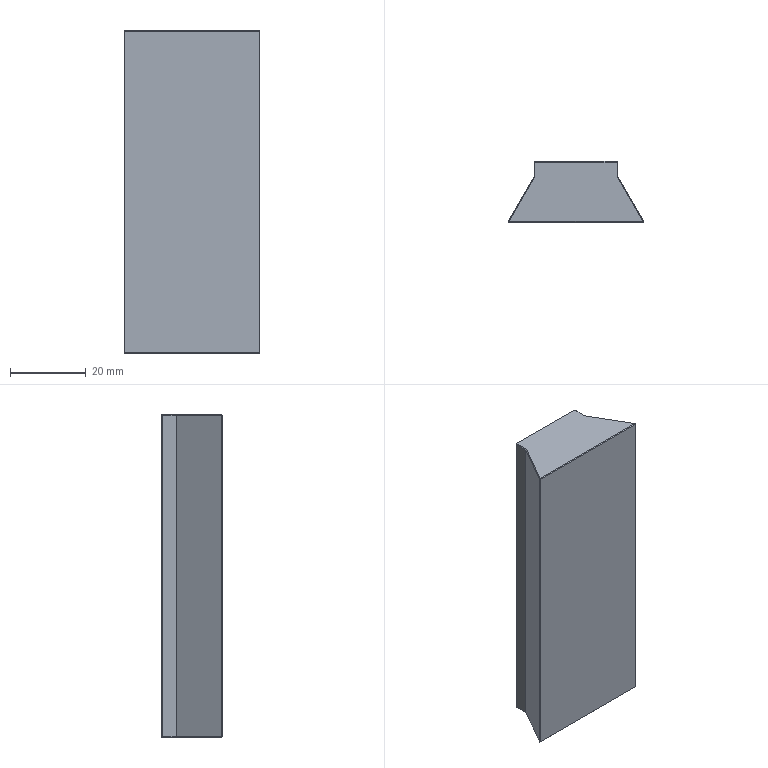Part | STEP file | 2007 | 1 solid | 24 faces | box 35.8 x 15.999 x 85 mm | volume 37123 mm3 | plane 24